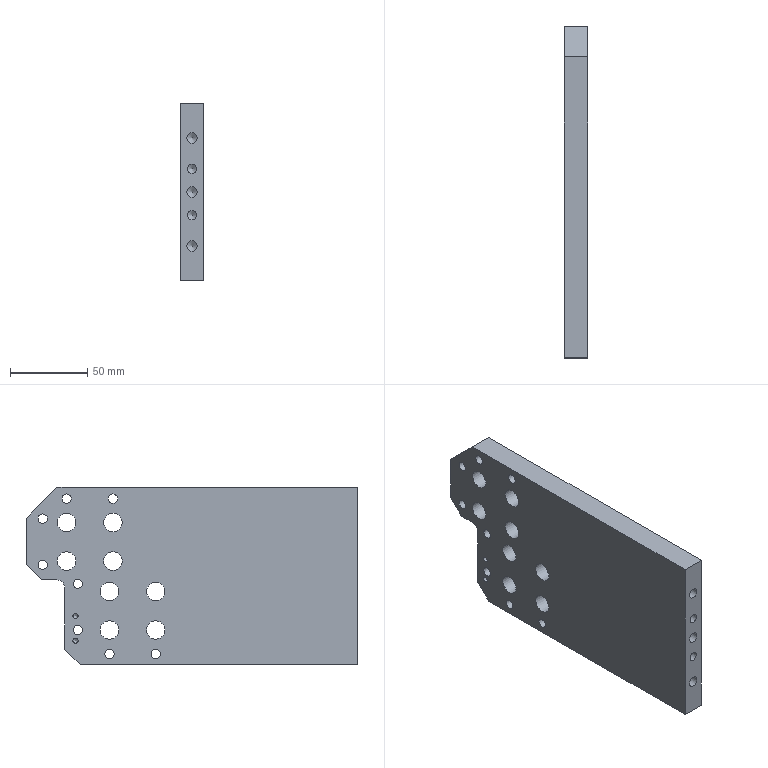Part | NX | features BREP 1 | 1 solid | 42 faces | box 15 x 215 x 115 mm | volume 325749 mm3 | cylinder 24 | plane 11 | cone 7 | commonest cylinder face diameters 6 x10 12 x8 6.8 x3 3.3 x2 10 x1
STEP:
#1=CARTESIAN_POINT('',(-7.5,-107.5,-57.5));
#2=VERTEX_POINT('',#1);
#3=CARTESIAN_POINT('',(-7.5,72.5,-57.5));
#4=VERTEX_POINT('',#3);
#5=CARTESIAN_POINT('',(-7.5,-107.5,-57.5));
#6=DIRECTION('',(0.,1.,0.));
#7=VECTOR('',#6,1000.);
#8=LINE('',#5,#7);
#9=EDGE_CURVE('',#2,#4,#8,.T.);
#10=ORIENTED_EDGE('',*,*,#9,.T.);
#11=CARTESIAN_POINT('',(7.5,72.5,-57.5));
#12=VERTEX_POINT('',#11);
#13=CARTESIAN_POINT('',(7.5,72.5,-57.5));
#14=DIRECTION('',(1.,0.,0.));
#15=VECTOR('',#14,1000.);
#16=LINE('',#13,#15);
#17=EDGE_CURVE('',#4,#12,#16,.T.);
#18=ORIENTED_EDGE('',*,*,#17,.T.);
#19=CARTESIAN_POINT('',(7.5,-107.5,-57.5));
#20=VERTEX_POINT('',#19);
#21=CARTESIAN_POINT('',(7.5,-107.5,-57.5));
#22=DIRECTION('',(0.,1.,0.));
#23=VECTOR('',#22,1000.);
#24=LINE('',#21,#23);
#25=EDGE_CURVE('',#20,#12,#24,.T.);
#26=ORIENTED_EDGE('',*,*,#25,.F.);
#27=CARTESIAN_POINT('',(7.5,-107.5,-57.5));
#28=DIRECTION('',(-1.,0.,0.));
#29=VECTOR('',#28,1000.);
#30=LINE('',#27,#29);
#31=EDGE_CURVE('',#20,#2,#30,.T.);
#32=ORIENTED_EDGE('',*,*,#31,.T.);
#33=EDGE_LOOP('',(#10,#18,#26,#32));
#34=FACE_BOUND('',#33,.T.);
#35=CARTESIAN_POINT('',(7.5,-107.5,-57.5));
#36=DIRECTION('',(0.,0.,1.));
#37=DIRECTION('',(-1.,0.,0.));
#38=AXIS2_PLACEMENT_3D('',#35,#36,#37);
#39=PLANE('',#38);
#40=ADVANCED_FACE('',(#34),#39,.F.);
#41=CARTESIAN_POINT('',(7.5,107.5,7.5));
#42=VERTEX_POINT('',#41);
#43=CARTESIAN_POINT('',(7.5,107.5,37.5));
#44=VERTEX_POINT('',#43);
#45=CARTESIAN_POINT('',(7.5,107.5,57.5));
#46=DIRECTION('',(0.,0.,1.));
#47=VECTOR('',#46,1000.);
#48=LINE('',#45,#47);
#49=EDGE_CURVE('',#42,#44,#48,.T.);
#50=ORIENTED_EDGE('',*,*,#49,.F.);
#51=CARTESIAN_POINT('',(-7.5,107.5,7.5));
#52=VERTEX_POINT('',#51);
#53=CARTESIAN_POINT('',(7.5,107.5,7.5));
#54=DIRECTION('',(-1.,0.,0.));
#55=VECTOR('',#54,1000.);
#56=LINE('',#53,#55);
#57=EDGE_CURVE('',#42,#52,#56,.T.);
#58=ORIENTED_EDGE('',*,*,#57,.T.);
#59=CARTESIAN_POINT('',(-7.5,107.5,37.5));
#60=VERTEX_POINT('',#59);
#61=CARTESIAN_POINT('',(-7.5,107.5,57.5));
#62=DIRECTION('',(0.,0.,1.));
#63=VECTOR('',#62,1000.);
#64=LINE('',#61,#63);
#65=EDGE_CURVE('',#52,#60,#64,.T.);
#66=ORIENTED_EDGE('',*,*,#65,.T.);
#67=CARTESIAN_POINT('',(7.5,107.5,37.5));
#68=DIRECTION('',(1.,0.,0.));
#69=VECTOR('',#68,1000.);
#70=LINE('',#67,#69);
#71=EDGE_CURVE('',#60,#44,#70,.T.);
#72=ORIENTED_EDGE('',*,*,#71,.T.);
#73=EDGE_LOOP('',(#50,#58,#66,#72));
#74=FACE_BOUND('',#73,.T.);
#75=CARTESIAN_POINT('',(7.5,107.5,57.5));
#76=DIRECTION('',(0.,-1.,0.));
#77=DIRECTION('',(0.,0.,1.));
#78=AXIS2_PLACEMENT_3D('',#75,#76,#77);
#79=PLANE('',#78);
#80=ADVANCED_FACE('',(#74),#79,.F.);
#81=CARTESIAN_POINT('',(7.5,87.5,57.5));
#82=VERTEX_POINT('',#81);
#83=CARTESIAN_POINT('',(7.5,-107.5,57.5));
#84=VERTEX_POINT('',#83);
#85=CARTESIAN_POINT('',(7.5,-107.5,57.5));
#86=DIRECTION('',(0.,-1.,0.));
#87=VECTOR('',#86,1000.);
#88=LINE('',#85,#87);
#89=EDGE_CURVE('',#82,#84,#88,.T.);
#90=ORIENTED_EDGE('',*,*,#89,.F.);
#91=CARTESIAN_POINT('',(-7.5,87.5,57.5));
#92=VERTEX_POINT('',#91);
#93=CARTESIAN_POINT('',(7.5,87.5,57.5));
#94=DIRECTION('',(-1.,0.,0.));
#95=VECTOR('',#94,1000.);
#96=LINE('',#93,#95);
#97=EDGE_CURVE('',#82,#92,#96,.T.);
#98=ORIENTED_EDGE('',*,*,#97,.T.);
#99=CARTESIAN_POINT('',(-7.5,-107.5,57.5));
#100=VERTEX_POINT('',#99);
#101=CARTESIAN_POINT('',(-7.5,-107.5,57.5));
#102=DIRECTION('',(0.,-1.,0.));
#103=VECTOR('',#102,1000.);
#104=LINE('',#101,#103);
#105=EDGE_CURVE('',#92,#100,#104,.T.);
#106=ORIENTED_EDGE('',*,*,#105,.T.);
#107=CARTESIAN_POINT('',(7.5,-107.5,57.5));
#108=DIRECTION('',(-1.,0.,0.));
#109=VECTOR('',#108,1000.);
#110=LINE('',#107,#109);
#111=EDGE_CURVE('',#84,#100,#110,.T.);
#112=ORIENTED_EDGE('',*,*,#111,.F.);
#113=EDGE_LOOP('',(#90,#98,#106,#112));
#114=FACE_BOUND('',#113,.T.);
#115=CARTESIAN_POINT('',(7.5,-107.5,57.5));
#116=DIRECTION('',(0.,0.,-1.));
#117=DIRECTION('',(1.,0.,0.));
#118=AXIS2_PLACEMENT_3D('',#115,#116,#117);
#119=PLANE('',#118);
#120=ADVANCED_FACE('',(#114),#119,.F.);
#121=CARTESIAN_POINT('',(0.,-107.5,-18.));
#122=VERTEX_POINT('',#121);
#123=CARTESIAN_POINT('',(0.,-107.5,-15.));
#124=DIRECTION('',(0.,-1.,0.));
#125=DIRECTION('',(0.,0.,-1.));
#126=AXIS2_PLACEMENT_3D('',#123,#124,#125);
#127=CIRCLE('',#126,3.);
#128=EDGE_CURVE('',#122,#122,#127,.T.);
#129=ORIENTED_EDGE('',*,*,#128,.F.);
#130=EDGE_LOOP('',(#129));
#131=FACE_BOUND('',#130,.T.);
#132=CARTESIAN_POINT('',(0.,-107.5,12.));
#133=VERTEX_POINT('',#132);
#134=CARTESIAN_POINT('',(0.,-107.5,15.));
#135=DIRECTION('',(0.,-1.,0.));
#136=DIRECTION('',(0.,0.,-1.));
#137=AXIS2_PLACEMENT_3D('',#134,#135,#136);
#138=CIRCLE('',#137,3.);
#139=EDGE_CURVE('',#133,#133,#138,.T.);
#140=ORIENTED_EDGE('',*,*,#139,.F.);
#141=EDGE_LOOP('',(#140));
#142=FACE_BOUND('',#141,.T.);
#143=CARTESIAN_POINT('',(0.,-107.5,31.6));
#144=VERTEX_POINT('',#143);
#145=CARTESIAN_POINT('',(0.,-107.5,35.));
#146=DIRECTION('',(0.,-1.,0.));
#147=DIRECTION('',(0.,0.,-1.));
#148=AXIS2_PLACEMENT_3D('',#145,#146,#147);
#149=CIRCLE('',#148,3.4);
#150=EDGE_CURVE('',#144,#144,#149,.T.);
#151=ORIENTED_EDGE('',*,*,#150,.F.);
#152=EDGE_LOOP('',(#151));
#153=FACE_BOUND('',#152,.T.);
#154=CARTESIAN_POINT('',(0.,-107.5,-38.4));
#155=VERTEX_POINT('',#154);
#156=CARTESIAN_POINT('',(0.,-107.5,-35.));
#157=DIRECTION('',(0.,-1.,0.));
#158=DIRECTION('',(0.,0.,-1.));
#159=AXIS2_PLACEMENT_3D('',#156,#157,#158);
#160=CIRCLE('',#159,3.4);
#161=EDGE_CURVE('',#155,#155,#160,.T.);
#162=ORIENTED_EDGE('',*,*,#161,.F.);
#163=EDGE_LOOP('',(#162));
#164=FACE_BOUND('',#163,.T.);
#165=CARTESIAN_POINT('',(0.,-107.5,-3.4));
#166=VERTEX_POINT('',#165);
#167=CARTESIAN_POINT('',(0.,-107.5,0.));
#168=DIRECTION('',(0.,-1.,0.));
#169=DIRECTION('',(0.,0.,-1.));
#170=AXIS2_PLACEMENT_3D('',#167,#168,#169);
#171=CIRCLE('',#170,3.4);
#172=EDGE_CURVE('',#166,#166,#171,.T.);
#173=ORIENTED_EDGE('',*,*,#172,.F.);
#174=EDGE_LOOP('',(#173));
#175=FACE_BOUND('',#174,.T.);
#176=CARTESIAN_POINT('',(-7.5,-107.5,57.5));
#177=DIRECTION('',(0.,0.,-1.));
#178=VECTOR('',#177,1000.);
#179=LINE('',#176,#178);
#180=EDGE_CURVE('',#100,#2,#179,.T.);
#181=ORIENTED_EDGE('',*,*,#180,.T.);
#182=ORIENTED_EDGE('',*,*,#31,.F.);
#183=CARTESIAN_POINT('',(7.5,-107.5,57.5));
#184=DIRECTION('',(0.,0.,-1.));
#185=VECTOR('',#184,1000.);
#186=LINE('',#183,#185);
#187=EDGE_CURVE('',#84,#20,#186,.T.);
#188=ORIENTED_EDGE('',*,*,#187,.F.);
#189=ORIENTED_EDGE('',*,*,#111,.T.);
#190=EDGE_LOOP('',(#181,#182,#188,#189));
#191=FACE_BOUND('',#190,.T.);
#192=CARTESIAN_POINT('',(7.5,-107.5,57.5));
#193=DIRECTION('',(0.,1.,0.));
#194=DIRECTION('',(0.,0.,-1.));
#195=AXIS2_PLACEMENT_3D('',#192,#193,#194);
#196=PLANE('',#195);
#197=ADVANCED_FACE('',(#131,#142,#153,#164,#175,#191),#196,.F.);
#198=CARTESIAN_POINT('',(7.5,53.5,-53.5));
#199=VERTEX_POINT('',#198);
#200=CARTESIAN_POINT('',(7.5,53.5,-50.5));
#201=DIRECTION('',(1.,0.,0.));
#202=DIRECTION('',(0.,0.,-1.));
#203=AXIS2_PLACEMENT_3D('',#200,#201,#202);
#204=CIRCLE('',#203,3.);
#205=EDGE_CURVE('',#199,#199,#204,.T.);
#206=ORIENTED_EDGE('',*,*,#205,.F.);
#207=EDGE_LOOP('',(#206));
#208=FACE_BOUND('',#207,.T.);
#209=CARTESIAN_POINT('',(7.5,23.5,-53.5));
#210=VERTEX_POINT('',#209);
#211=CARTESIAN_POINT('',(7.5,23.5,-50.5));
#212=DIRECTION('',(1.,0.,0.));
#213=DIRECTION('',(0.,0.,-1.));
#214=AXIS2_PLACEMENT_3D('',#211,#212,#213);
#215=CIRCLE('',#214,3.);
#216=EDGE_CURVE('',#210,#210,#215,.T.);
#217=ORIENTED_EDGE('',*,*,#216,.F.);
#218=EDGE_LOOP('',(#217));
#219=FACE_BOUND('',#218,.T.);
#220=CARTESIAN_POINT('',(7.5,74.,-38.));
#221=VERTEX_POINT('',#220);
#222=CARTESIAN_POINT('',(7.5,74.,-35.));
#223=DIRECTION('',(1.,0.,0.));
#224=DIRECTION('',(0.,0.,-1.));
#225=AXIS2_PLACEMENT_3D('',#222,#223,#224);
#226=CIRCLE('',#225,3.);
#227=EDGE_CURVE('',#221,#221,#226,.T.);
#228=ORIENTED_EDGE('',*,*,#227,.F.);
#229=EDGE_LOOP('',(#228));
#230=FACE_BOUND('',#229,.T.);
#231=CARTESIAN_POINT('',(7.5,74.,-8.));
#232=VERTEX_POINT('',#231);
#233=CARTESIAN_POINT('',(7.5,74.,-5.));
#234=DIRECTION('',(1.,0.,0.));
#235=DIRECTION('',(0.,0.,-1.));
#236=AXIS2_PLACEMENT_3D('',#233,#234,#235);
#237=CIRCLE('',#236,3.);
#238=EDGE_CURVE('',#232,#232,#237,.T.);
#239=ORIENTED_EDGE('',*,*,#238,.F.);
#240=EDGE_LOOP('',(#239));
#241=FACE_BOUND('',#240,.T.);
#242=CARTESIAN_POINT('',(7.5,96.75,4.2));
#243=VERTEX_POINT('',#242);
#244=CARTESIAN_POINT('',(7.5,96.75,7.2));
#245=DIRECTION('',(1.,0.,0.));
#246=DIRECTION('',(0.,0.,-1.));
#247=AXIS2_PLACEMENT_3D('',#244,#245,#246);
#248=CIRCLE('',#247,3.);
#249=EDGE_CURVE('',#243,#243,#248,.T.);
#250=ORIENTED_EDGE('',*,*,#249,.F.);
#251=EDGE_LOOP('',(#250));
#252=FACE_BOUND('',#251,.T.);
#253=CARTESIAN_POINT('',(7.5,96.75,34.2));
#254=VERTEX_POINT('',#253);
#255=CARTESIAN_POINT('',(7.5,96.75,37.2));
#256=DIRECTION('',(1.,0.,0.));
#257=DIRECTION('',(0.,0.,-1.));
#258=AXIS2_PLACEMENT_3D('',#255,#256,#257);
#259=CIRCLE('',#258,3.);
#260=EDGE_CURVE('',#254,#254,#259,.T.);
#261=ORIENTED_EDGE('',*,*,#260,.F.);
#262=EDGE_LOOP('',(#261));
#263=FACE_BOUND('',#262,.T.);
#264=CARTESIAN_POINT('',(7.5,81.25,47.2));
#265=VERTEX_POINT('',#264);
#266=CARTESIAN_POINT('',(7.5,81.25,50.2));
#267=DIRECTION('',(1.,0.,0.));
#268=DIRECTION('',(0.,0.,-1.));
#269=AXIS2_PLACEMENT_3D('',#266,#267,#268);
#270=CIRCLE('',#269,3.);
#271=EDGE_CURVE('',#265,#265,#270,.T.);
#272=ORIENTED_EDGE('',*,*,#271,.F.);
#273=EDGE_LOOP('',(#272));
#274=FACE_BOUND('',#273,.T.);
#275=CARTESIAN_POINT('',(7.5,51.25,47.2));
#276=VERTEX_POINT('',#275);
#277=CARTESIAN_POINT('',(7.5,51.25,50.2));
#278=DIRECTION('',(1.,0.,0.));
#279=DIRECTION('',(0.,0.,-1.));
#280=AXIS2_PLACEMENT_3D('',#277,#278,#279);
#281=CIRCLE('',#280,3.);
#282=EDGE_CURVE('',#276,#276,#281,.T.);
#283=ORIENTED_EDGE('',*,*,#282,.F.);
#284=EDGE_LOOP('',(#283));
#285=FACE_BOUND('',#284,.T.);
#286=CARTESIAN_POINT('',(7.5,23.5,-29.));
#287=VERTEX_POINT('',#286);
#288=CARTESIAN_POINT('',(7.5,23.5,-35.));
#289=DIRECTION('',(-1.,0.,0.));
#290=DIRECTION('',(0.,0.,1.));
#291=AXIS2_PLACEMENT_3D('',#288,#289,#290);
#292=CIRCLE('',#291,6.);
#293=EDGE_CURVE('',#287,#287,#292,.T.);
#294=ORIENTED_EDGE('',*,*,#293,.T.);
#295=EDGE_LOOP('',(#294));
#296=FACE_BOUND('',#295,.T.);
#297=CARTESIAN_POINT('',(7.5,23.5,-4.));
#298=VERTEX_POINT('',#297);
#299=CARTESIAN_POINT('',(7.5,23.5,-10.));
#300=DIRECTION('',(-1.,0.,0.));
#301=DIRECTION('',(0.,0.,1.));
#302=AXIS2_PLACEMENT_3D('',#299,#300,#301);
#303=CIRCLE('',#302,6.);
#304=EDGE_CURVE('',#298,#298,#303,.T.);
#305=ORIENTED_EDGE('',*,*,#304,.T.);
#306=EDGE_LOOP('',(#305));
#307=FACE_BOUND('',#306,.T.);
#308=CARTESIAN_POINT('',(7.5,53.5,-29.));
#309=VERTEX_POINT('',#308);
#310=CARTESIAN_POINT('',(7.5,53.5,-35.));
#311=DIRECTION('',(-1.,0.,0.));
#312=DIRECTION('',(0.,0.,1.));
#313=AXIS2_PLACEMENT_3D('',#310,#311,#312);
#314=CIRCLE('',#313,6.);
#315=EDGE_CURVE('',#309,#309,#314,.T.);
#316=ORIENTED_EDGE('',*,*,#315,.T.);
#317=EDGE_LOOP('',(#316));
#318=FACE_BOUND('',#317,.T.);
#319=CARTESIAN_POINT('',(7.5,53.5,-4.));
#320=VERTEX_POINT('',#319);
#321=CARTESIAN_POINT('',(7.5,53.5,-10.));
#322=DIRECTION('',(-1.,0.,0.));
#323=DIRECTION('',(0.,0.,1.));
#324=AXIS2_PLACEMENT_3D('',#321,#322,#323);
#325=CIRCLE('',#324,6.);
#326=EDGE_CURVE('',#320,#320,#325,.T.);
#327=ORIENTED_EDGE('',*,*,#326,.T.);
#328=EDGE_LOOP('',(#327));
#329=FACE_BOUND('',#328,.T.);
#330=CARTESIAN_POINT('',(7.5,81.25,15.7));
#331=VERTEX_POINT('',#330);
#332=CARTESIAN_POINT('',(7.5,81.25,9.7));
#333=DIRECTION('',(-1.,0.,0.));
#334=DIRECTION('',(0.,0.,1.));
#335=AXIS2_PLACEMENT_3D('',#332,#333,#334);
#336=CIRCLE('',#335,6.);
#337=EDGE_CURVE('',#331,#331,#336,.T.);
#338=ORIENTED_EDGE('',*,*,#337,.T.);
#339=EDGE_LOOP('',(#338));
#340=FACE_BOUND('',#339,.T.);
#341=CARTESIAN_POINT('',(7.5,51.25,40.7));
#342=VERTEX_POINT('',#341);
#343=CARTESIAN_POINT('',(7.5,51.25,34.7));
#344=DIRECTION('',(-1.,0.,0.));
#345=DIRECTION('',(0.,0.,1.));
#346=AXIS2_PLACEMENT_3D('',#343,#344,#345);
#347=CIRCLE('',#346,6.);
#348=EDGE_CURVE('',#342,#342,#347,.T.);
#349=ORIENTED_EDGE('',*,*,#348,.T.);
#350=EDGE_LOOP('',(#349));
#351=FACE_BOUND('',#350,.T.);
#352=CARTESIAN_POINT('',(7.5,51.25,15.7));
#353=VERTEX_POINT('',#352);
#354=CARTESIAN_POINT('',(7.5,51.25,9.7));
#355=DIRECTION('',(-1.,0.,0.));
#356=DIRECTION('',(0.,0.,1.));
#357=AXIS2_PLACEMENT_3D('',#354,#355,#356);
#358=CIRCLE('',#357,6.);
#359=EDGE_CURVE('',#353,#353,#358,.T.);
#360=ORIENTED_EDGE('',*,*,#359,.T.);
#361=EDGE_LOOP('',(#360));
#362=FACE_BOUND('',#361,.T.);
#363=CARTESIAN_POINT('',(7.5,81.25,40.7));
#364=VERTEX_POINT('',#363);
#365=CARTESIAN_POINT('',(7.5,81.25,34.7));
#366=DIRECTION('',(-1.,0.,0.));
#367=DIRECTION('',(0.,0.,1.));
#368=AXIS2_PLACEMENT_3D('',#365,#366,#367);
#369=CIRCLE('',#368,6.);
#370=EDGE_CURVE('',#364,#364,#369,.T.);
#371=ORIENTED_EDGE('',*,*,#370,.T.);
#372=EDGE_LOOP('',(#371));
#373=FACE_BOUND('',#372,.T.);
#374=CARTESIAN_POINT('',(7.5,97.5,-2.5));
#375=VERTEX_POINT('',#374);
#376=CARTESIAN_POINT('',(7.5,87.5,-2.5));
#377=VERTEX_POINT('',#376);
#378=CARTESIAN_POINT('',(7.5,107.5,-2.5));
#379=DIRECTION('',(0.,-1.,0.));
#380=VECTOR('',#379,1000.);
#381=LINE('',#378,#380);
#382=EDGE_CURVE('',#375,#377,#381,.T.);
#383=ORIENTED_EDGE('',*,*,#382,.F.);
#384=CARTESIAN_POINT('',(7.5,107.5,7.5));
#385=DIRECTION('',(0.,0.7071,0.7071));
#386=VECTOR('',#385,1000.);
#387=LINE('',#384,#386);
#388=EDGE_CURVE('',#375,#42,#387,.T.);
#389=ORIENTED_EDGE('',*,*,#388,.T.);
#390=ORIENTED_EDGE('',*,*,#49,.T.);
#391=CARTESIAN_POINT('',(7.5,87.5,57.5));
#392=DIRECTION('',(0.,-0.7071,0.7071));
#393=VECTOR('',#392,1000.);
#394=LINE('',#391,#393);
#395=EDGE_CURVE('',#44,#82,#394,.T.);
#396=ORIENTED_EDGE('',*,*,#395,.T.);
#397=ORIENTED_EDGE('',*,*,#89,.T.);
#398=ORIENTED_EDGE('',*,*,#187,.T.);
#399=ORIENTED_EDGE('',*,*,#25,.T.);
#400=CARTESIAN_POINT('',(7.5,82.5,-47.5));
#401=VERTEX_POINT('',#400);
#402=CARTESIAN_POINT('',(7.5,82.5,-47.5));
#403=DIRECTION('',(0.,0.7071,0.7071));
#404=VECTOR('',#403,1000.);
#405=LINE('',#402,#404);
#406=EDGE_CURVE('',#12,#401,#405,.T.);
#407=ORIENTED_EDGE('',*,*,#406,.T.);
#408=CARTESIAN_POINT('',(7.5,82.5,-7.5));
#409=VERTEX_POINT('',#408);
#410=CARTESIAN_POINT('',(7.5,82.5,-2.5));
#411=DIRECTION('',(0.,0.,-1.));
#412=VECTOR('',#411,1000.);
#413=LINE('',#410,#412);
#414=EDGE_CURVE('',#409,#401,#413,.T.);
#415=ORIENTED_EDGE('',*,*,#414,.F.);
#416=CARTESIAN_POINT('',(7.5,87.5,-7.5));
#417=DIRECTION('',(-1.,0.,0.));
#418=DIRECTION('',(0.,0.,1.));
#419=AXIS2_PLACEMENT_3D('',#416,#417,#418);
#420=CIRCLE('',#419,5.);
#421=EDGE_CURVE('',#409,#377,#420,.T.);
#422=ORIENTED_EDGE('',*,*,#421,.T.);
#423=EDGE_LOOP('',(#383,#389,#390,#396,#397,#398,#399,#407,#415,#422));
#424=FACE_BOUND('',#423,.T.);
#425=CARTESIAN_POINT('',(7.5,0.,0.));
#426=DIRECTION('',(-1.,0.,0.));
#427=DIRECTION('',(0.,0.,-1.));
#428=AXIS2_PLACEMENT_3D('',#425,#426,#427);
#429=PLANE('',#428);
#430=ADVANCED_FACE('',(#208,#219,#230,#241,#252,#263,#274,#285,#296,#307,#318,#329,#340,#351,#362,#373,#424),#429,.F.);
#431=CARTESIAN_POINT('',(-7.5,75.5,-40.298));
#432=VERTEX_POINT('',#431);
#433=CARTESIAN_POINT('',(-7.5,75.5,-41.948));
#434=DIRECTION('',(-1.,0.,0.));
#435=DIRECTION('',(0.,0.,1.));
#436=AXIS2_PLACEMENT_3D('',#433,#434,#435);
#437=CIRCLE('',#436,1.65);
#438=EDGE_CURVE('',#432,#432,#437,.T.);
#439=ORIENTED_EDGE('',*,*,#438,.F.);
#440=EDGE_LOOP('',(#439));
#441=FACE_BOUND('',#440,.T.);
#442=CARTESIAN_POINT('',(-7.5,75.5,-24.298));
#443=VERTEX_POINT('',#442);
#444=CARTESIAN_POINT('',(-7.5,75.5,-25.948));
#445=DIRECTION('',(-1.,0.,0.));
#446=DIRECTION('',(0.,0.,1.));
#447=AXIS2_PLACEMENT_3D('',#444,#445,#446);
#448=CIRCLE('',#447,1.65);
#449=EDGE_CURVE('',#443,#443,#448,.T.);
#450=ORIENTED_EDGE('',*,*,#449,.F.);
#451=EDGE_LOOP('',(#450));
#452=FACE_BOUND('',#451,.T.);
#453=ORIENTED_EDGE('',*,*,#65,.F.);
#454=CARTESIAN_POINT('',(-7.5,97.5,-2.5));
#455=VERTEX_POINT('',#454);
#456=CARTESIAN_POINT('',(-7.5,50.,-50.));
#457=DIRECTION('',(0.,-0.7071,-0.7071));
#458=VECTOR('',#457,1000.);
#459=LINE('',#456,#458);
#460=EDGE_CURVE('',#52,#455,#459,.T.);
#461=ORIENTED_EDGE('',*,*,#460,.T.);
#462=CARTESIAN_POINT('',(-7.5,87.5,-2.5));
#463=VERTEX_POINT('',#462);
#464=CARTESIAN_POINT('',(-7.5,107.5,-2.5));
#465=DIRECTION('',(0.,1.,0.));
#466=VECTOR('',#465,1000.);
#467=LINE('',#464,#466);
#468=EDGE_CURVE('',#463,#455,#467,.T.);
#469=ORIENTED_EDGE('',*,*,#468,.F.);
#470=CARTESIAN_POINT('',(-7.5,82.5,-7.5));
#471=VERTEX_POINT('',#470);
#472=CARTESIAN_POINT('',(-7.5,87.5,-7.5));
#473=DIRECTION('',(1.,0.,0.));
#474=DIRECTION('',(0.,0.,1.));
#475=AXIS2_PLACEMENT_3D('',#472,#473,#474);
#476=CIRCLE('',#475,5.);
#477=EDGE_CURVE('',#463,#471,#476,.T.);
#478=ORIENTED_EDGE('',*,*,#477,.T.);
#479=CARTESIAN_POINT('',(-7.5,82.5,-47.5));
#480=VERTEX_POINT('',#479);
#481=CARTESIAN_POINT('',(-7.5,82.5,-2.5));
#482=DIRECTION('',(0.,0.,1.));
#483=VECTOR('',#482,1000.);
#484=LINE('',#481,#483);
#485=EDGE_CURVE('',#480,#471,#484,.T.);
#486=ORIENTED_EDGE('',*,*,#485,.F.);
#487=CARTESIAN_POINT('',(-7.5,65.,-65.));
#488=DIRECTION('',(0.,-0.7071,-0.7071));
#489=VECTOR('',#488,1000.);
#490=LINE('',#487,#489);
#491=EDGE_CURVE('',#480,#4,#490,.T.);
#492=ORIENTED_EDGE('',*,*,#491,.T.);
#493=ORIENTED_EDGE('',*,*,#9,.F.);
#494=ORIENTED_EDGE('',*,*,#180,.F.);
#495=ORIENTED_EDGE('',*,*,#105,.F.);
#496=CARTESIAN_POINT('',(-7.5,72.5,72.5));
#497=DIRECTION('',(0.,0.7071,-0.7071));
#498=VECTOR('',#497,1000.);
#499=LINE('',#496,#498);
#500=EDGE_CURVE('',#92,#60,#499,.T.);
#501=ORIENTED_EDGE('',*,*,#500,.T.);
#502=EDGE_LOOP('',(#453,#461,#469,#478,#486,#492,#493,#494,#495,#501));
#503=FACE_BOUND('',#502,.T.);
#504=CARTESIAN_POINT('',(-7.5,53.5,-53.5));
#505=VERTEX_POINT('',#504);
#506=CARTESIAN_POINT('',(-7.5,53.5,-50.5));
#507=DIRECTION('',(1.,0.,0.));
#508=DIRECTION('',(0.,0.,-1.));
#509=AXIS2_PLACEMENT_3D('',#506,#507,#508);
#510=CIRCLE('',#509,3.);
#511=EDGE_CURVE('',#505,#505,#510,.T.);
#512=ORIENTED_EDGE('',*,*,#511,.T.);
#513=EDGE_LOOP('',(#512));
#514=FACE_BOUND('',#513,.T.);
#515=CARTESIAN_POINT('',(-7.5,23.5,-53.5));
#516=VERTEX_POINT('',#515);
#517=CARTESIAN_POINT('',(-7.5,23.5,-50.5));
#518=DIRECTION('',(1.,0.,0.));
#519=DIRECTION('',(0.,0.,-1.));
#520=AXIS2_PLACEMENT_3D('',#517,#518,#519);
#521=CIRCLE('',#520,3.);
#522=EDGE_CURVE('',#516,#516,#521,.T.);
#523=ORIENTED_EDGE('',*,*,#522,.T.);
#524=EDGE_LOOP('',(#523));
#525=FACE_BOUND('',#524,.T.);
#526=CARTESIAN_POINT('',(-7.5,74.,-38.));
#527=VERTEX_POINT('',#526);
#528=CARTESIAN_POINT('',(-7.5,74.,-35.));
#529=DIRECTION('',(1.,0.,0.));
#530=DIRECTION('',(0.,0.,-1.));
#531=AXIS2_PLACEMENT_3D('',#528,#529,#530);
#532=CIRCLE('',#531,3.);
#533=EDGE_CURVE('',#527,#527,#532,.T.);
#534=ORIENTED_EDGE('',*,*,#533,.T.);
#535=EDGE_LOOP('',(#534));
#536=FACE_BOUND('',#535,.T.);
#537=CARTESIAN_POINT('',(-7.5,74.,-8.));
#538=VERTEX_POINT('',#537);
#539=CARTESIAN_POINT('',(-7.5,74.,-5.));
#540=DIRECTION('',(1.,0.,0.));
#541=DIRECTION('',(0.,0.,-1.));
#542=AXIS2_PLACEMENT_3D('',#539,#540,#541);
#543=CIRCLE('',#542,3.);
#544=EDGE_CURVE('',#538,#538,#543,.T.);
#545=ORIENTED_EDGE('',*,*,#544,.T.);
#546=EDGE_LOOP('',(#545));
#547=FACE_BOUND('',#546,.T.);
#548=CARTESIAN_POINT('',(-7.5,96.75,4.2));
#549=VERTEX_POINT('',#548);
#550=CARTESIAN_POINT('',(-7.5,96.75,7.2));
#551=DIRECTION('',(1.,0.,0.));
#552=DIRECTION('',(0.,0.,-1.));
#553=AXIS2_PLACEMENT_3D('',#550,#551,#552);
#554=CIRCLE('',#553,3.);
#555=EDGE_CURVE('',#549,#549,#554,.T.);
#556=ORIENTED_EDGE('',*,*,#555,.T.);
#557=EDGE_LOOP('',(#556));
#558=FACE_BOUND('',#557,.T.);
#559=CARTESIAN_POINT('',(-7.5,96.75,34.2));
#560=VERTEX_POINT('',#559);
#561=CARTESIAN_POINT('',(-7.5,96.75,37.2));
#562=DIRECTION('',(1.,0.,0.));
#563=DIRECTION('',(0.,0.,-1.));
#564=AXIS2_PLACEMENT_3D('',#561,#562,#563);
#565=CIRCLE('',#564,3.);
#566=EDGE_CURVE('',#560,#560,#565,.T.);
#567=ORIENTED_EDGE('',*,*,#566,.T.);
#568=EDGE_LOOP('',(#567));
#569=FACE_BOUND('',#568,.T.);
#570=CARTESIAN_POINT('',(-7.5,81.25,47.2));
#571=VERTEX_POINT('',#570);
#572=CARTESIAN_POINT('',(-7.5,81.25,50.2));
#573=DIRECTION('',(1.,0.,0.));
#574=DIRECTION('',(0.,0.,-1.));
#575=AXIS2_PLACEMENT_3D('',#572,#573,#574);
#576=CIRCLE('',#575,3.);
#577=EDGE_CURVE('',#571,#571,#576,.T.);
#578=ORIENTED_EDGE('',*,*,#577,.T.);
#579=EDGE_LOOP('',(#578));
#580=FACE_BOUND('',#579,.T.);
#581=CARTESIAN_POINT('',(-7.5,51.25,47.2));
#582=VERTEX_POINT('',#581);
#583=CARTESIAN_POINT('',(-7.5,51.25,50.2));
#584=DIRECTION('',(1.,0.,0.));
#585=DIRECTION('',(0.,0.,-1.));
#586=AXIS2_PLACEMENT_3D('',#583,#584,#585);
#587=CIRCLE('',#586,3.);
#588=EDGE_CURVE('',#582,#582,#587,.T.);
#589=ORIENTED_EDGE('',*,*,#588,.T.);
#590=EDGE_LOOP('',(#589));
#591=FACE_BOUND('',#590,.T.);
#592=CARTESIAN_POINT('',(-7.5,23.5,-29.));
#593=VERTEX_POINT('',#592);
#594=CARTESIAN_POINT('',(-7.5,23.5,-35.));
#595=DIRECTION('',(-1.,0.,0.));
#596=DIRECTION('',(0.,0.,1.));
#597=AXIS2_PLACEMENT_3D('',#594,#595,#596);
#598=CIRCLE('',#597,6.);
#599=EDGE_CURVE('',#593,#593,#598,.T.);
#600=ORIENTED_EDGE('',*,*,#599,.F.);
#601=EDGE_LOOP('',(#600));
#602=FACE_BOUND('',#601,.T.);
#603=CARTESIAN_POINT('',(-7.5,23.5,-4.));
#604=VERTEX_POINT('',#603);
#605=CARTESIAN_POINT('',(-7.5,23.5,-10.));
#606=DIRECTION('',(-1.,0.,0.));
#607=DIRECTION('',(0.,0.,1.));
#608=AXIS2_PLACEMENT_3D('',#605,#606,#607);
#609=CIRCLE('',#608,6.);
#610=EDGE_CURVE('',#604,#604,#609,.T.);
#611=ORIENTED_EDGE('',*,*,#610,.F.);
#612=EDGE_LOOP('',(#611));
#613=FACE_BOUND('',#612,.T.);
#614=CARTESIAN_POINT('',(-7.5,53.5,-29.));
#615=VERTEX_POINT('',#614);
#616=CARTESIAN_POINT('',(-7.5,53.5,-35.));
#617=DIRECTION('',(-1.,0.,0.));
#618=DIRECTION('',(0.,0.,1.));
#619=AXIS2_PLACEMENT_3D('',#616,#617,#618);
#620=CIRCLE('',#619,6.);
#621=EDGE_CURVE('',#615,#615,#620,.T.);
#622=ORIENTED_EDGE('',*,*,#621,.F.);
#623=EDGE_LOOP('',(#622));
#624=FACE_BOUND('',#623,.T.);
#625=CARTESIAN_POINT('',(-7.5,53.5,-4.));
#626=VERTEX_POINT('',#625);
#627=CARTESIAN_POINT('',(-7.5,53.5,-10.));
#628=DIRECTION('',(-1.,0.,0.));
#629=DIRECTION('',(0.,0.,1.));
#630=AXIS2_PLACEMENT_3D('',#627,#628,#629);
#631=CIRCLE('',#630,6.);
#632=EDGE_CURVE('',#626,#626,#631,.T.);
#633=ORIENTED_EDGE('',*,*,#632,.F.);
#634=EDGE_LOOP('',(#633));
#635=FACE_BOUND('',#634,.T.);
#636=CARTESIAN_POINT('',(-7.5,81.25,15.7));
#637=VERTEX_POINT('',#636);
#638=CARTESIAN_POINT('',(-7.5,81.25,9.7));
#639=DIRECTION('',(-1.,0.,0.));
#640=DIRECTION('',(0.,0.,1.));
#641=AXIS2_PLACEMENT_3D('',#638,#639,#640);
#642=CIRCLE('',#641,6.);
#643=EDGE_CURVE('',#637,#637,#642,.T.);
#644=ORIENTED_EDGE('',*,*,#643,.F.);
#645=EDGE_LOOP('',(#644));
#646=FACE_BOUND('',#645,.T.);
#647=CARTESIAN_POINT('',(-7.5,51.25,40.7));
#648=VERTEX_POINT('',#647);
#649=CARTESIAN_POINT('',(-7.5,51.25,34.7));
#650=DIRECTION('',(-1.,0.,0.));
#651=DIRECTION('',(0.,0.,1.));
#652=AXIS2_PLACEMENT_3D('',#649,#650,#651);
#653=CIRCLE('',#652,6.);
#654=EDGE_CURVE('',#648,#648,#653,.T.);
#655=ORIENTED_EDGE('',*,*,#654,.F.);
#656=EDGE_LOOP('',(#655));
#657=FACE_BOUND('',#656,.T.);
#658=CARTESIAN_POINT('',(-7.5,51.25,15.7));
#659=VERTEX_POINT('',#658);
#660=CARTESIAN_POINT('',(-7.5,51.25,9.7));
#661=DIRECTION('',(-1.,0.,0.));
#662=DIRECTION('',(0.,0.,1.));
#663=AXIS2_PLACEMENT_3D('',#660,#661,#662);
#664=CIRCLE('',#663,6.);
#665=EDGE_CURVE('',#659,#659,#664,.T.);
#666=ORIENTED_EDGE('',*,*,#665,.F.);
#667=EDGE_LOOP('',(#666));
#668=FACE_BOUND('',#667,.T.);
#669=CARTESIAN_POINT('',(-7.5,81.25,40.7));
#670=VERTEX_POINT('',#669);
#671=CARTESIAN_POINT('',(-7.5,81.25,34.7));
#672=DIRECTION('',(-1.,0.,0.));
#673=DIRECTION('',(0.,0.,1.));
#674=AXIS2_PLACEMENT_3D('',#671,#672,#673);
#675=CIRCLE('',#674,6.);
#676=EDGE_CURVE('',#670,#670,#675,.T.);
#677=ORIENTED_EDGE('',*,*,#676,.F.);
#678=EDGE_LOOP('',(#677));
#679=FACE_BOUND('',#678,.T.);
#680=CARTESIAN_POINT('',(-7.5,0.,0.));
#681=DIRECTION('',(-1.,0.,0.));
#682=DIRECTION('',(0.,0.,-1.));
#683=AXIS2_PLACEMENT_3D('',#680,#681,#682);
#684=PLANE('',#683);
#685=ADVANCED_FACE('',(#441,#452,#503,#514,#525,#536,#547,#558,#569,#580,#591,#602,#613,#624,#635,#646,#657,#668,#679),#684,.T.);
#686=ORIENTED_EDGE('',*,*,#370,.F.);
#687=EDGE_LOOP('',(#686));
#688=FACE_BOUND('',#687,.T.);
#689=ORIENTED_EDGE('',*,*,#676,.T.);
#690=EDGE_LOOP('',(#689));
#691=FACE_BOUND('',#690,.T.);
#692=CARTESIAN_POINT('',(-7.5,81.25,34.7));
#693=DIRECTION('',(-1.,0.,0.));
#694=DIRECTION('',(0.,0.,-1.));
#695=AXIS2_PLACEMENT_3D('',#692,#693,#694);
#696=CYLINDRICAL_SURFACE('',#695,6.);
#697=ADVANCED_FACE('',(#688,#691),#696,.F.);
#698=ORIENTED_EDGE('',*,*,#359,.F.);
#699=EDGE_LOOP('',(#698));
#700=FACE_BOUND('',#699,.T.);
#701=ORIENTED_EDGE('',*,*,#665,.T.);
#702=EDGE_LOOP('',(#701));
#703=FACE_BOUND('',#702,.T.);
#704=CARTESIAN_POINT('',(-7.5,51.25,9.7));
#705=DIRECTION('',(-1.,0.,0.));
#706=DIRECTION('',(0.,0.,-1.));
#707=AXIS2_PLACEMENT_3D('',#704,#705,#706);
#708=CYLINDRICAL_SURFACE('',#707,6.);
#709=ADVANCED_FACE('',(#700,#703),#708,.F.);
#710=ORIENTED_EDGE('',*,*,#348,.F.);
#711=EDGE_LOOP('',(#710));
#712=FACE_BOUND('',#711,.T.);
#713=ORIENTED_EDGE('',*,*,#654,.T.);
#714=EDGE_LOOP('',(#713));
#715=FACE_BOUND('',#714,.T.);
#716=CARTESIAN_POINT('',(-7.5,51.25,34.7));
#717=DIRECTION('',(-1.,0.,0.));
#718=DIRECTION('',(0.,0.,-1.));
#719=AXIS2_PLACEMENT_3D('',#716,#717,#718);
#720=CYLINDRICAL_SURFACE('',#719,6.);
#721=ADVANCED_FACE('',(#712,#715),#720,.F.);
#722=ORIENTED_EDGE('',*,*,#337,.F.);
#723=EDGE_LOOP('',(#722));
#724=FACE_BOUND('',#723,.T.);
#725=ORIENTED_EDGE('',*,*,#643,.T.);
#726=EDGE_LOOP('',(#725));
#727=FACE_BOUND('',#726,.T.);
#728=CARTESIAN_POINT('',(-7.5,81.25,9.7));
#729=DIRECTION('',(-1.,0.,0.));
#730=DIRECTION('',(0.,0.,-1.));
#731=AXIS2_PLACEMENT_3D('',#728,#729,#730);
#732=CYLINDRICAL_SURFACE('',#731,6.);
#733=ADVANCED_FACE('',(#724,#727),#732,.F.);
#734=ORIENTED_EDGE('',*,*,#326,.F.);
#735=EDGE_LOOP('',(#734));
#736=FACE_BOUND('',#735,.T.);
#737=ORIENTED_EDGE('',*,*,#632,.T.);
#738=EDGE_LOOP('',(#737));
#739=FACE_BOUND('',#738,.T.);
#740=CARTESIAN_POINT('',(-7.5,53.5,-10.));
#741=DIRECTION('',(-1.,0.,0.));
#742=DIRECTION('',(0.,0.,-1.));
#743=AXIS2_PLACEMENT_3D('',#740,#741,#742);
#744=CYLINDRICAL_SURFACE('',#743,6.);
#745=ADVANCED_FACE('',(#736,#739),#744,.F.);
#746=ORIENTED_EDGE('',*,*,#315,.F.);
#747=EDGE_LOOP('',(#746));
#748=FACE_BOUND('',#747,.T.);
#749=ORIENTED_EDGE('',*,*,#621,.T.);
#750=EDGE_LOOP('',(#749));
#751=FACE_BOUND('',#750,.T.);
#752=CARTESIAN_POINT('',(-7.5,53.5,-35.));
#753=DIRECTION('',(-1.,0.,0.));
#754=DIRECTION('',(0.,0.,-1.));
#755=AXIS2_PLACEMENT_3D('',#752,#753,#754);
#756=CYLINDRICAL_SURFACE('',#755,6.);
#757=ADVANCED_FACE('',(#748,#751),#756,.F.);
#758=ORIENTED_EDGE('',*,*,#304,.F.);
#759=EDGE_LOOP('',(#758));
#760=FACE_BOUND('',#759,.T.);
#761=ORIENTED_EDGE('',*,*,#610,.T.);
#762=EDGE_LOOP('',(#761));
#763=FACE_BOUND('',#762,.T.);
#764=CARTESIAN_POINT('',(-7.5,23.5,-10.));
#765=DIRECTION('',(-1.,0.,0.));
#766=DIRECTION('',(0.,0.,-1.));
#767=AXIS2_PLACEMENT_3D('',#764,#765,#766);
#768=CYLINDRICAL_SURFACE('',#767,6.);
#769=ADVANCED_FACE('',(#760,#763),#768,.F.);
#770=ORIENTED_EDGE('',*,*,#293,.F.);
#771=EDGE_LOOP('',(#770));
#772=FACE_BOUND('',#771,.T.);
#773=ORIENTED_EDGE('',*,*,#599,.T.);
#774=EDGE_LOOP('',(#773));
#775=FACE_BOUND('',#774,.T.);
#776=CARTESIAN_POINT('',(-7.5,23.5,-35.));
#777=DIRECTION('',(-1.,0.,0.));
#778=DIRECTION('',(0.,0.,-1.));
#779=AXIS2_PLACEMENT_3D('',#776,#777,#778);
#780=CYLINDRICAL_SURFACE('',#779,6.);
#781=ADVANCED_FACE('',(#772,#775),#780,.F.);
#782=ORIENTED_EDGE('',*,*,#588,.F.);
#783=EDGE_LOOP('',(#782));
#784=FACE_BOUND('',#783,.T.);
#785=ORIENTED_EDGE('',*,*,#282,.T.);
#786=EDGE_LOOP('',(#785));
#787=FACE_BOUND('',#786,.T.);
#788=CARTESIAN_POINT('',(7.5,51.25,50.2));
#789=DIRECTION('',(1.,0.,0.));
#790=DIRECTION('',(0.,0.,1.));
#791=AXIS2_PLACEMENT_3D('',#788,#789,#790);
#792=CYLINDRICAL_SURFACE('',#791,3.);
#793=ADVANCED_FACE('',(#784,#787),#792,.F.);
#794=ORIENTED_EDGE('',*,*,#577,.F.);
#795=EDGE_LOOP('',(#794));
#796=FACE_BOUND('',#795,.T.);
#797=ORIENTED_EDGE('',*,*,#271,.T.);
#798=EDGE_LOOP('',(#797));
#799=FACE_BOUND('',#798,.T.);
#800=CARTESIAN_POINT('',(7.5,81.25,50.2));
#801=DIRECTION('',(1.,0.,0.));
#802=DIRECTION('',(0.,0.,1.));
#803=AXIS2_PLACEMENT_3D('',#800,#801,#802);
#804=CYLINDRICAL_SURFACE('',#803,3.);
#805=ADVANCED_FACE('',(#796,#799),#804,.F.);
#806=ORIENTED_EDGE('',*,*,#566,.F.);
#807=EDGE_LOOP('',(#806));
#808=FACE_BOUND('',#807,.T.);
#809=ORIENTED_EDGE('',*,*,#260,.T.);
#810=EDGE_LOOP('',(#809));
#811=FACE_BOUND('',#810,.T.);
#812=CARTESIAN_POINT('',(7.5,96.75,37.2));
#813=DIRECTION('',(1.,0.,0.));
#814=DIRECTION('',(0.,0.,1.));
#815=AXIS2_PLACEMENT_3D('',#812,#813,#814);
#816=CYLINDRICAL_SURFACE('',#815,3.);
#817=ADVANCED_FACE('',(#808,#811),#816,.F.);
#818=ORIENTED_EDGE('',*,*,#555,.F.);
#819=EDGE_LOOP('',(#818));
#820=FACE_BOUND('',#819,.T.);
#821=ORIENTED_EDGE('',*,*,#249,.T.);
#822=EDGE_LOOP('',(#821));
#823=FACE_BOUND('',#822,.T.);
#824=CARTESIAN_POINT('',(7.5,96.75,7.2));
#825=DIRECTION('',(1.,0.,0.));
#826=DIRECTION('',(0.,0.,1.));
#827=AXIS2_PLACEMENT_3D('',#824,#825,#826);
#828=CYLINDRICAL_SURFACE('',#827,3.);
#829=ADVANCED_FACE('',(#820,#823),#828,.F.);
#830=ORIENTED_EDGE('',*,*,#544,.F.);
#831=EDGE_LOOP('',(#830));
#832=FACE_BOUND('',#831,.T.);
#833=ORIENTED_EDGE('',*,*,#238,.T.);
#834=EDGE_LOOP('',(#833));
#835=FACE_BOUND('',#834,.T.);
#836=CARTESIAN_POINT('',(7.5,74.,-5.));
#837=DIRECTION('',(1.,0.,0.));
#838=DIRECTION('',(0.,0.,1.));
#839=AXIS2_PLACEMENT_3D('',#836,#837,#838);
#840=CYLINDRICAL_SURFACE('',#839,3.);
#841=ADVANCED_FACE('',(#832,#835),#840,.F.);
#842=ORIENTED_EDGE('',*,*,#533,.F.);
#843=EDGE_LOOP('',(#842));
#844=FACE_BOUND('',#843,.T.);
#845=ORIENTED_EDGE('',*,*,#227,.T.);
#846=EDGE_LOOP('',(#845));
#847=FACE_BOUND('',#846,.T.);
#848=CARTESIAN_POINT('',(7.5,74.,-35.));
#849=DIRECTION('',(1.,0.,0.));
#850=DIRECTION('',(0.,0.,1.));
#851=AXIS2_PLACEMENT_3D('',#848,#849,#850);
#852=CYLINDRICAL_SURFACE('',#851,3.);
#853=ADVANCED_FACE('',(#844,#847),#852,.F.);
#854=ORIENTED_EDGE('',*,*,#522,.F.);
#855=EDGE_LOOP('',(#854));
#856=FACE_BOUND('',#855,.T.);
#857=ORIENTED_EDGE('',*,*,#216,.T.);
#858=EDGE_LOOP('',(#857));
#859=FACE_BOUND('',#858,.T.);
#860=CARTESIAN_POINT('',(7.5,23.5,-50.5));
#861=DIRECTION('',(1.,0.,0.));
#862=DIRECTION('',(0.,0.,1.));
#863=AXIS2_PLACEMENT_3D('',#860,#861,#862);
#864=CYLINDRICAL_SURFACE('',#863,3.);
#865=ADVANCED_FACE('',(#856,#859),#864,.F.);
#866=ORIENTED_EDGE('',*,*,#511,.F.);
#867=EDGE_LOOP('',(#866));
#868=FACE_BOUND('',#867,.T.);
#869=ORIENTED_EDGE('',*,*,#205,.T.);
#870=EDGE_LOOP('',(#869));
#871=FACE_BOUND('',#870,.T.);
#872=CARTESIAN_POINT('',(7.5,53.5,-50.5));
#873=DIRECTION('',(1.,0.,0.));
#874=DIRECTION('',(0.,0.,1.));
#875=AXIS2_PLACEMENT_3D('',#872,#873,#874);
#876=CYLINDRICAL_SURFACE('',#875,3.);
#877=ADVANCED_FACE('',(#868,#871),#876,.F.);
#878=CARTESIAN_POINT('',(0.,-85.707,0.));
#879=VERTEX_POINT('',#878);
#880=VERTEX_LOOP('',#879);
#881=FACE_BOUND('',#880,.T.);
#882=CARTESIAN_POINT('',(0.,-87.75,-3.4));
#883=VERTEX_POINT('',#882);
#884=CARTESIAN_POINT('',(0.,-87.75,0.));
#885=DIRECTION('',(0.,-1.,0.));
#886=DIRECTION('',(0.,0.,-1.));
#887=AXIS2_PLACEMENT_3D('',#884,#885,#886);
#888=CIRCLE('',#887,3.4);
#889=EDGE_CURVE('',#883,#883,#888,.T.);
#890=ORIENTED_EDGE('',*,*,#889,.T.);
#891=EDGE_LOOP('',(#890));
#892=FACE_BOUND('',#891,.T.);
#893=CARTESIAN_POINT('',(0.,-87.75,0.));
#894=DIRECTION('',(0.,-1.,0.));
#895=DIRECTION('',(0.,0.,1.));
#896=AXIS2_PLACEMENT_3D('',#893,#894,#895);
#897=CONICAL_SURFACE('',#896,3.4,1.03);
#898=ADVANCED_FACE('',(#881,#892),#897,.F.);
#899=ORIENTED_EDGE('',*,*,#889,.F.);
#900=EDGE_LOOP('',(#899));
#901=FACE_BOUND('',#900,.T.);
#902=ORIENTED_EDGE('',*,*,#172,.T.);
#903=EDGE_LOOP('',(#902));
#904=FACE_BOUND('',#903,.T.);
#905=CARTESIAN_POINT('',(0.,-107.5,0.));
#906=DIRECTION('',(0.,-1.,0.));
#907=DIRECTION('',(0.,0.,1.));
#908=AXIS2_PLACEMENT_3D('',#905,#906,#907);
#909=CYLINDRICAL_SURFACE('',#908,3.4);
#910=ADVANCED_FACE('',(#901,#904),#909,.F.);
#911=CARTESIAN_POINT('',(0.,-85.707,-35.));
#912=VERTEX_POINT('',#911);
#913=VERTEX_LOOP('',#912);
#914=FACE_BOUND('',#913,.T.);
#915=CARTESIAN_POINT('',(0.,-87.75,-38.4));
#916=VERTEX_POINT('',#915);
#917=CARTESIAN_POINT('',(0.,-87.75,-35.));
#918=DIRECTION('',(0.,-1.,0.));
#919=DIRECTION('',(0.,0.,-1.));
#920=AXIS2_PLACEMENT_3D('',#917,#918,#919);
#921=CIRCLE('',#920,3.4);
#922=EDGE_CURVE('',#916,#916,#921,.T.);
#923=ORIENTED_EDGE('',*,*,#922,.T.);
#924=EDGE_LOOP('',(#923));
#925=FACE_BOUND('',#924,.T.);
#926=CARTESIAN_POINT('',(0.,-87.75,-35.));
#927=DIRECTION('',(0.,-1.,0.));
#928=DIRECTION('',(0.,0.,1.));
#929=AXIS2_PLACEMENT_3D('',#926,#927,#928);
#930=CONICAL_SURFACE('',#929,3.4,1.03);
#931=ADVANCED_FACE('',(#914,#925),#930,.F.);
#932=ORIENTED_EDGE('',*,*,#922,.F.);
#933=EDGE_LOOP('',(#932));
#934=FACE_BOUND('',#933,.T.);
#935=ORIENTED_EDGE('',*,*,#161,.T.);
#936=EDGE_LOOP('',(#935));
#937=FACE_BOUND('',#936,.T.);
#938=CARTESIAN_POINT('',(0.,-107.5,-35.));
#939=DIRECTION('',(0.,-1.,0.));
#940=DIRECTION('',(0.,0.,1.));
#941=AXIS2_PLACEMENT_3D('',#938,#939,#940);
#942=CYLINDRICAL_SURFACE('',#941,3.4);
#943=ADVANCED_FACE('',(#934,#937),#942,.F.);
#944=CARTESIAN_POINT('',(0.,-85.707,35.));
#945=VERTEX_POINT('',#944);
#946=VERTEX_LOOP('',#945);
#947=FACE_BOUND('',#946,.T.);
#948=CARTESIAN_POINT('',(0.,-87.75,31.6));
#949=VERTEX_POINT('',#948);
#950=CARTESIAN_POINT('',(0.,-87.75,35.));
#951=DIRECTION('',(0.,-1.,0.));
#952=DIRECTION('',(0.,0.,-1.));
#953=AXIS2_PLACEMENT_3D('',#950,#951,#952);
#954=CIRCLE('',#953,3.4);
#955=EDGE_CURVE('',#949,#949,#954,.T.);
#956=ORIENTED_EDGE('',*,*,#955,.T.);
#957=EDGE_LOOP('',(#956));
#958=FACE_BOUND('',#957,.T.);
#959=CARTESIAN_POINT('',(0.,-87.75,35.));
#960=DIRECTION('',(0.,-1.,0.));
#961=DIRECTION('',(0.,0.,1.));
#962=AXIS2_PLACEMENT_3D('',#959,#960,#961);
#963=CONICAL_SURFACE('',#962,3.4,1.03);
#964=ADVANCED_FACE('',(#947,#958),#963,.F.);
#965=ORIENTED_EDGE('',*,*,#955,.F.);
#966=EDGE_LOOP('',(#965));
#967=FACE_BOUND('',#966,.T.);
#968=ORIENTED_EDGE('',*,*,#150,.T.);
#969=EDGE_LOOP('',(#968));
#970=FACE_BOUND('',#969,.T.);
#971=CARTESIAN_POINT('',(0.,-107.5,35.));
#972=DIRECTION('',(0.,-1.,0.));
#973=DIRECTION('',(0.,0.,1.));
#974=AXIS2_PLACEMENT_3D('',#971,#972,#973);
#975=CYLINDRICAL_SURFACE('',#974,3.4);
#976=ADVANCED_FACE('',(#967,#970),#975,.F.);
#977=CARTESIAN_POINT('',(0.,-93.697,15.));
#978=VERTEX_POINT('',#977);
#979=VERTEX_LOOP('',#978);
#980=FACE_BOUND('',#979,.T.);
#981=CARTESIAN_POINT('',(0.,-95.5,12.));
#982=VERTEX_POINT('',#981);
#983=CARTESIAN_POINT('',(0.,-95.5,15.));
#984=DIRECTION('',(0.,-1.,0.));
#985=DIRECTION('',(0.,0.,-1.));
#986=AXIS2_PLACEMENT_3D('',#983,#984,#985);
#987=CIRCLE('',#986,3.);
#988=EDGE_CURVE('',#982,#982,#987,.T.);
#989=ORIENTED_EDGE('',*,*,#988,.T.);
#990=EDGE_LOOP('',(#989));
#991=FACE_BOUND('',#990,.T.);
#992=CARTESIAN_POINT('',(0.,-95.5,15.));
#993=DIRECTION('',(0.,-1.,0.));
#994=DIRECTION('',(0.,0.,1.));
#995=AXIS2_PLACEMENT_3D('',#992,#993,#994);
#996=CONICAL_SURFACE('',#995,3.,1.03);
#997=ADVANCED_FACE('',(#980,#991),#996,.F.);
#998=ORIENTED_EDGE('',*,*,#988,.F.);
#999=EDGE_LOOP('',(#998));
#1000=FACE_BOUND('',#999,.T.);
#1001=ORIENTED_EDGE('',*,*,#139,.T.);
#1002=EDGE_LOOP('',(#1001));
#1003=FACE_BOUND('',#1002,.T.);
#1004=CARTESIAN_POINT('',(0.,-107.5,15.));
#1005=DIRECTION('',(0.,-1.,0.));
#1006=DIRECTION('',(0.,0.,1.));
#1007=AXIS2_PLACEMENT_3D('',#1004,#1005,#1006);
#1008=CYLINDRICAL_SURFACE('',#1007,3.);
#1009=ADVANCED_FACE('',(#1000,#1003),#1008,.F.);
#1010=CARTESIAN_POINT('',(0.,-93.697,-15.));
#1011=VERTEX_POINT('',#1010);
#1012=VERTEX_LOOP('',#1011);
#1013=FACE_BOUND('',#1012,.T.);
#1014=CARTESIAN_POINT('',(0.,-95.5,-18.));
#1015=VERTEX_POINT('',#1014);
#1016=CARTESIAN_POINT('',(0.,-95.5,-15.));
#1017=DIRECTION('',(0.,-1.,0.));
#1018=DIRECTION('',(0.,0.,-1.));
#1019=AXIS2_PLACEMENT_3D('',#1016,#1017,#1018);
#1020=CIRCLE('',#1019,3.);
#1021=EDGE_CURVE('',#1015,#1015,#1020,.T.);
#1022=ORIENTED_EDGE('',*,*,#1021,.T.);
#1023=EDGE_LOOP('',(#1022));
#1024=FACE_BOUND('',#1023,.T.);
#1025=CARTESIAN_POINT('',(0.,-95.5,-15.));
#1026=DIRECTION('',(0.,-1.,0.));
#1027=DIRECTION('',(0.,0.,1.));
#1028=AXIS2_PLACEMENT_3D('',#1025,#1026,#1027);
#1029=CONICAL_SURFACE('',#1028,3.,1.03);
#1030=ADVANCED_FACE('',(#1013,#1024),#1029,.F.);
#1031=ORIENTED_EDGE('',*,*,#1021,.F.);
#1032=EDGE_LOOP('',(#1031));
#1033=FACE_BOUND('',#1032,.T.);
#1034=ORIENTED_EDGE('',*,*,#128,.T.);
#1035=EDGE_LOOP('',(#1034));
#1036=FACE_BOUND('',#1035,.T.);
#1037=CARTESIAN_POINT('',(0.,-107.5,-15.));
#1038=DIRECTION('',(0.,-1.,0.));
#1039=DIRECTION('',(0.,0.,1.));
#1040=AXIS2_PLACEMENT_3D('',#1037,#1038,#1039);
#1041=CYLINDRICAL_SURFACE('',#1040,3.);
#1042=ADVANCED_FACE('',(#1033,#1036),#1041,.F.);
#1043=ORIENTED_EDGE('',*,*,#395,.F.);
#1044=ORIENTED_EDGE('',*,*,#71,.F.);
#1045=ORIENTED_EDGE('',*,*,#500,.F.);
#1046=ORIENTED_EDGE('',*,*,#97,.F.);
#1047=EDGE_LOOP('',(#1043,#1044,#1045,#1046));
#1048=FACE_BOUND('',#1047,.T.);
#1049=CARTESIAN_POINT('',(7.5,87.5,57.5));
#1050=DIRECTION('',(0.,-0.7071,-0.7071));
#1051=DIRECTION('',(1.,0.,0.));
#1052=AXIS2_PLACEMENT_3D('',#1049,#1050,#1051);
#1053=PLANE('',#1052);
#1054=ADVANCED_FACE('',(#1048),#1053,.F.);
#1055=ORIENTED_EDGE('',*,*,#382,.T.);
#1056=CARTESIAN_POINT('',(-7.5,87.5,-2.5));
#1057=DIRECTION('',(-1.,0.,0.));
#1058=VECTOR('',#1057,1000.);
#1059=LINE('',#1056,#1058);
#1060=EDGE_CURVE('',#377,#463,#1059,.T.);
#1061=ORIENTED_EDGE('',*,*,#1060,.T.);
#1062=ORIENTED_EDGE('',*,*,#468,.T.);
#1063=CARTESIAN_POINT('',(67.915,97.5,-2.5));
#1064=DIRECTION('',(1.,0.,0.));
#1065=VECTOR('',#1064,1000.);
#1066=LINE('',#1063,#1065);
#1067=EDGE_CURVE('',#455,#375,#1066,.T.);
#1068=ORIENTED_EDGE('',*,*,#1067,.T.);
#1069=EDGE_LOOP('',(#1055,#1061,#1062,#1068));
#1070=FACE_BOUND('',#1069,.T.);
#1071=CARTESIAN_POINT('',(67.915,107.5,-2.5));
#1072=DIRECTION('',(0.,0.,1.));
#1073=DIRECTION('',(0.,1.,0.));
#1074=AXIS2_PLACEMENT_3D('',#1071,#1072,#1073);
#1075=PLANE('',#1074);
#1076=ADVANCED_FACE('',(#1070),#1075,.F.);
#1077=ORIENTED_EDGE('',*,*,#485,.T.);
#1078=CARTESIAN_POINT('',(7.5,82.5,-7.5));
#1079=DIRECTION('',(1.,0.,0.));
#1080=VECTOR('',#1079,1000.);
#1081=LINE('',#1078,#1080);
#1082=EDGE_CURVE('',#471,#409,#1081,.T.);
#1083=ORIENTED_EDGE('',*,*,#1082,.T.);
#1084=ORIENTED_EDGE('',*,*,#414,.T.);
#1085=CARTESIAN_POINT('',(67.915,82.5,-47.5));
#1086=DIRECTION('',(-1.,0.,0.));
#1087=VECTOR('',#1086,1000.);
#1088=LINE('',#1085,#1087);
#1089=EDGE_CURVE('',#401,#480,#1088,.T.);
#1090=ORIENTED_EDGE('',*,*,#1089,.T.);
#1091=EDGE_LOOP('',(#1077,#1083,#1084,#1090));
#1092=FACE_BOUND('',#1091,.T.);
#1093=CARTESIAN_POINT('',(67.915,82.5,-2.5));
#1094=DIRECTION('',(0.,-1.,0.));
#1095=DIRECTION('',(0.,0.,1.));
#1096=AXIS2_PLACEMENT_3D('',#1093,#1094,#1095);
#1097=PLANE('',#1096);
#1098=ADVANCED_FACE('',(#1092),#1097,.F.);
#1099=ORIENTED_EDGE('',*,*,#388,.F.);
#1100=ORIENTED_EDGE('',*,*,#1067,.F.);
#1101=ORIENTED_EDGE('',*,*,#460,.F.);
#1102=ORIENTED_EDGE('',*,*,#57,.F.);
#1103=EDGE_LOOP('',(#1099,#1100,#1101,#1102));
#1104=FACE_BOUND('',#1103,.T.);
#1105=CARTESIAN_POINT('',(7.5,107.5,7.5));
#1106=DIRECTION('',(0.,-0.7071,0.7071));
#1107=DIRECTION('',(1.,0.,0.));
#1108=AXIS2_PLACEMENT_3D('',#1105,#1106,#1107);
#1109=PLANE('',#1108);
#1110=ADVANCED_FACE('',(#1104),#1109,.F.);
#1111=ORIENTED_EDGE('',*,*,#406,.F.);
#1112=ORIENTED_EDGE('',*,*,#17,.F.);
#1113=ORIENTED_EDGE('',*,*,#491,.F.);
#1114=ORIENTED_EDGE('',*,*,#1089,.F.);
#1115=EDGE_LOOP('',(#1111,#1112,#1113,#1114));
#1116=FACE_BOUND('',#1115,.T.);
#1117=CARTESIAN_POINT('',(67.915,82.5,-47.5));
#1118=DIRECTION('',(0.,-0.7071,0.7071));
#1119=DIRECTION('',(1.,0.,0.));
#1120=AXIS2_PLACEMENT_3D('',#1117,#1118,#1119);
#1121=PLANE('',#1120);
#1122=ADVANCED_FACE('',(#1116),#1121,.F.);
#1123=ORIENTED_EDGE('',*,*,#421,.F.);
#1124=ORIENTED_EDGE('',*,*,#1082,.F.);
#1125=ORIENTED_EDGE('',*,*,#477,.F.);
#1126=ORIENTED_EDGE('',*,*,#1060,.F.);
#1127=EDGE_LOOP('',(#1123,#1124,#1125,#1126));
#1128=FACE_BOUND('',#1127,.T.);
#1129=CARTESIAN_POINT('',(67.915,87.5,-7.5));
#1130=DIRECTION('',(1.,0.,0.));
#1131=DIRECTION('',(0.,0.,1.));
#1132=AXIS2_PLACEMENT_3D('',#1129,#1130,#1131);
#1133=CYLINDRICAL_SURFACE('',#1132,5.);
#1134=ADVANCED_FACE('',(#1128),#1133,.F.);
#1135=CARTESIAN_POINT('',(3.591,75.5,-25.948));
#1136=VERTEX_POINT('',#1135);
#1137=VERTEX_LOOP('',#1136);
#1138=FACE_BOUND('',#1137,.T.);
#1139=CARTESIAN_POINT('',(2.6,75.5,-24.298));
#1140=VERTEX_POINT('',#1139);
#1141=CARTESIAN_POINT('',(2.6,75.5,-25.948));
#1142=DIRECTION('',(-1.,0.,0.));
#1143=DIRECTION('',(0.,0.,1.));
#1144=AXIS2_PLACEMENT_3D('',#1141,#1142,#1143);
#1145=CIRCLE('',#1144,1.65);
#1146=EDGE_CURVE('',#1140,#1140,#1145,.T.);
#1147=ORIENTED_EDGE('',*,*,#1146,.T.);
#1148=EDGE_LOOP('',(#1147));
#1149=FACE_BOUND('',#1148,.T.);
#1150=CARTESIAN_POINT('',(2.6,75.5,-25.948));
#1151=DIRECTION('',(-1.,0.,0.));
#1152=DIRECTION('',(0.,0.,-1.));
#1153=AXIS2_PLACEMENT_3D('',#1150,#1151,#1152);
#1154=CONICAL_SURFACE('',#1153,1.65,1.03);
#1155=ADVANCED_FACE('',(#1138,#1149),#1154,.F.);
#1156=ORIENTED_EDGE('',*,*,#1146,.F.);
#1157=EDGE_LOOP('',(#1156));
#1158=FACE_BOUND('',#1157,.T.);
#1159=ORIENTED_EDGE('',*,*,#449,.T.);
#1160=EDGE_LOOP('',(#1159));
#1161=FACE_BOUND('',#1160,.T.);
#1162=CARTESIAN_POINT('',(-7.5,75.5,-25.948));
#1163=DIRECTION('',(-1.,0.,0.));
#1164=DIRECTION('',(0.,0.,-1.));
#1165=AXIS2_PLACEMENT_3D('',#1162,#1163,#1164);
#1166=CYLINDRICAL_SURFACE('',#1165,1.65);
#1167=ADVANCED_FACE('',(#1158,#1161),#1166,.F.);
#1168=CARTESIAN_POINT('',(3.591,75.5,-41.948));
#1169=VERTEX_POINT('',#1168);
#1170=VERTEX_LOOP('',#1169);
#1171=FACE_BOUND('',#1170,.T.);
#1172=CARTESIAN_POINT('',(2.6,75.5,-40.298));
#1173=VERTEX_POINT('',#1172);
#1174=CARTESIAN_POINT('',(2.6,75.5,-41.948));
#1175=DIRECTION('',(-1.,0.,0.));
#1176=DIRECTION('',(0.,0.,1.));
#1177=AXIS2_PLACEMENT_3D('',#1174,#1175,#1176);
#1178=CIRCLE('',#1177,1.65);
#1179=EDGE_CURVE('',#1173,#1173,#1178,.T.);
#1180=ORIENTED_EDGE('',*,*,#1179,.T.);
#1181=EDGE_LOOP('',(#1180));
#1182=FACE_BOUND('',#1181,.T.);
#1183=CARTESIAN_POINT('',(2.6,75.5,-41.948));
#1184=DIRECTION('',(-1.,0.,0.));
#1185=DIRECTION('',(0.,0.,-1.));
#1186=AXIS2_PLACEMENT_3D('',#1183,#1184,#1185);
#1187=CONICAL_SURFACE('',#1186,1.65,1.03);
#1188=ADVANCED_FACE('',(#1171,#1182),#1187,.F.);
#1189=ORIENTED_EDGE('',*,*,#1179,.F.);
#1190=EDGE_LOOP('',(#1189));
#1191=FACE_BOUND('',#1190,.T.);
#1192=ORIENTED_EDGE('',*,*,#438,.T.);
#1193=EDGE_LOOP('',(#1192));
#1194=FACE_BOUND('',#1193,.T.);
#1195=CARTESIAN_POINT('',(-7.5,75.5,-41.948));
#1196=DIRECTION('',(-1.,0.,0.));
#1197=DIRECTION('',(0.,0.,-1.));
#1198=AXIS2_PLACEMENT_3D('',#1195,#1196,#1197);
#1199=CYLINDRICAL_SURFACE('',#1198,1.65);
#1200=ADVANCED_FACE('',(#1191,#1194),#1199,.F.);
#1201=CLOSED_SHELL('',(#40,#80,#120,#197,#430,#685,#697,#709,#721,#733,#745,#757,#769,#781,#793,#805,#817,#829,#841,#853,#865,#877,#898,#910,#931,#943,#964,#976,#997,#1009,#1030,#1042,#1054,#1076,#1098,#1110,#1122,#1134,#1155,#1167,#1188,#1200));
#1202=MANIFOLD_SOLID_BREP('',#1201);
#1203=(LENGTH_UNIT()NAMED_UNIT(*)SI_UNIT(.MILLI.,.METRE.));
#1204=UNCERTAINTY_MEASURE_WITH_UNIT(LENGTH_MEASURE(0.00001),#1203,'','');
#1205=(NAMED_UNIT(*)PLANE_ANGLE_UNIT()SI_UNIT($,.RADIAN.));
#1206=(NAMED_UNIT(*)SI_UNIT($,.STERADIAN.)SOLID_ANGLE_UNIT());
#1207=(GEOMETRIC_REPRESENTATION_CONTEXT(3)GLOBAL_UNCERTAINTY_ASSIGNED_CONTEXT((#1204))GLOBAL_UNIT_ASSIGNED_CONTEXT((#1203,#1205,#1206))REPRESENTATION_CONTEXT('',''));
#1208=ADVANCED_BREP_SHAPE_REPRESENTATION('',(#1202),#1207);